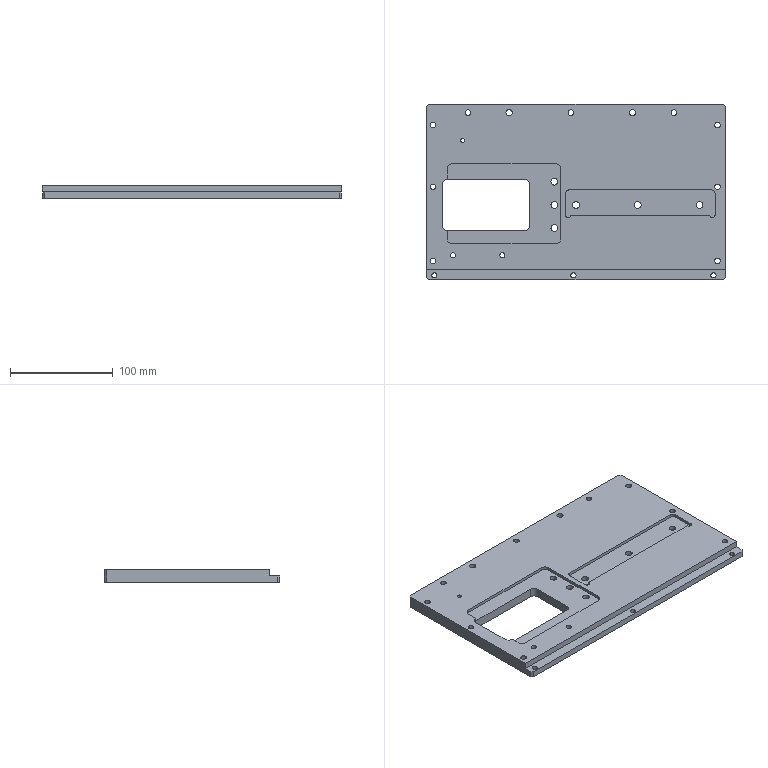Part | STEP file | J454-EBZ05-12-03-Part-1-4 | 1 solid | 130 faces | box 290 x 170 x 12 mm | volume 488791 mm3 | cylinder 88 | plane 42 | commonest cylinder face diameters 5.5 x18 9.5 x18 5 x12 6.6 x12 11 x12 10 x8